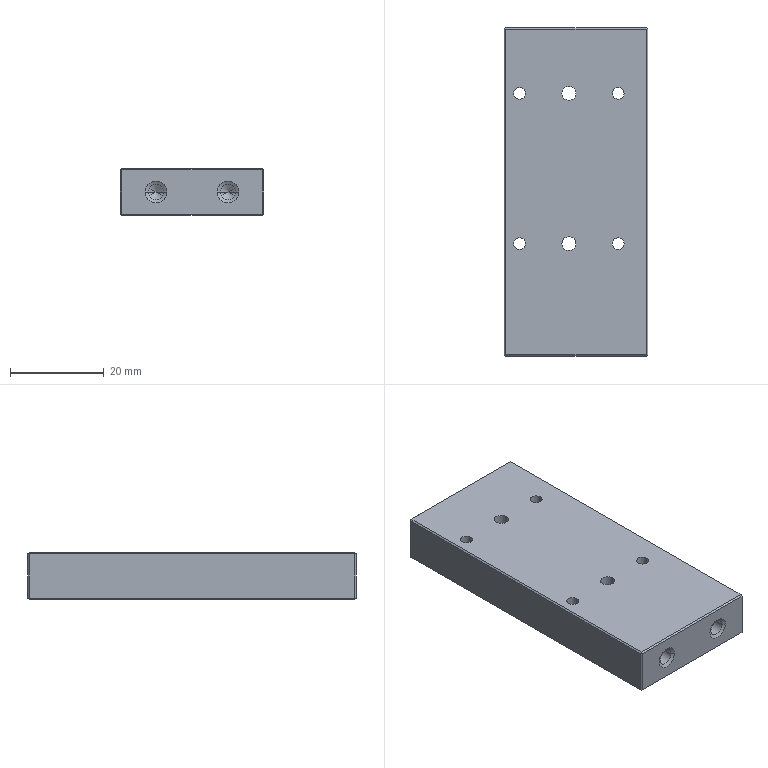Part | NX | 1 solid | 58 faces | box 30.6 x 70 x 10 mm | volume 20843 mm3 | cylinder 20 | cone 20 | plane 18 | commonest cylinder face diameters 2.5 x8 3.3 x8 3 x4